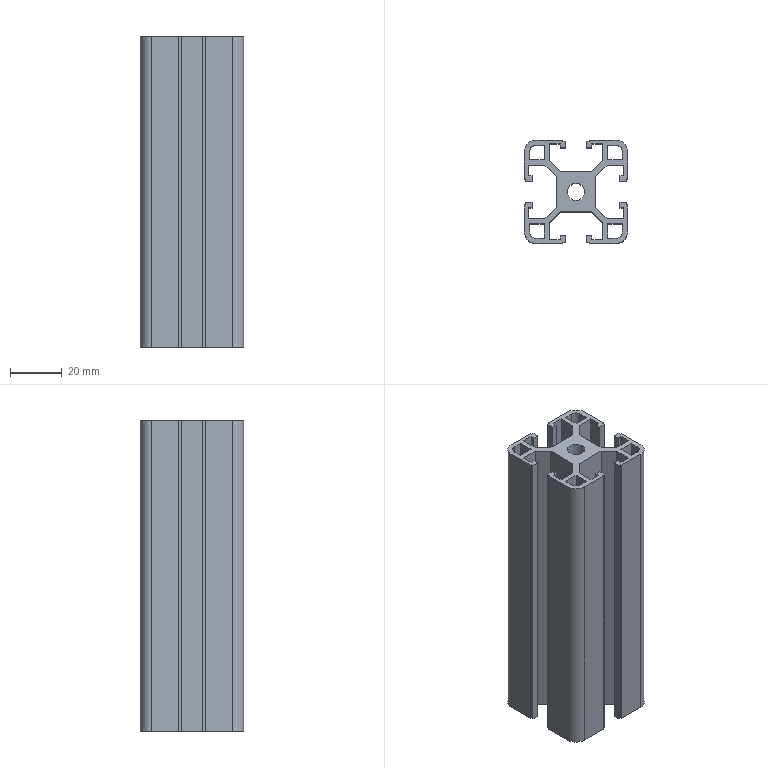Part | NX | features DATUM_CSYS 2, EXTRUDE 1, SKETCH 1 | 1 solid | 103 faces | box 40 x 40 x 120 mm | volume 69185 mm3 | plane 94 | cylinder 9 | commonest cylinder face diameters 5 x4 9 x4 6.8 x1